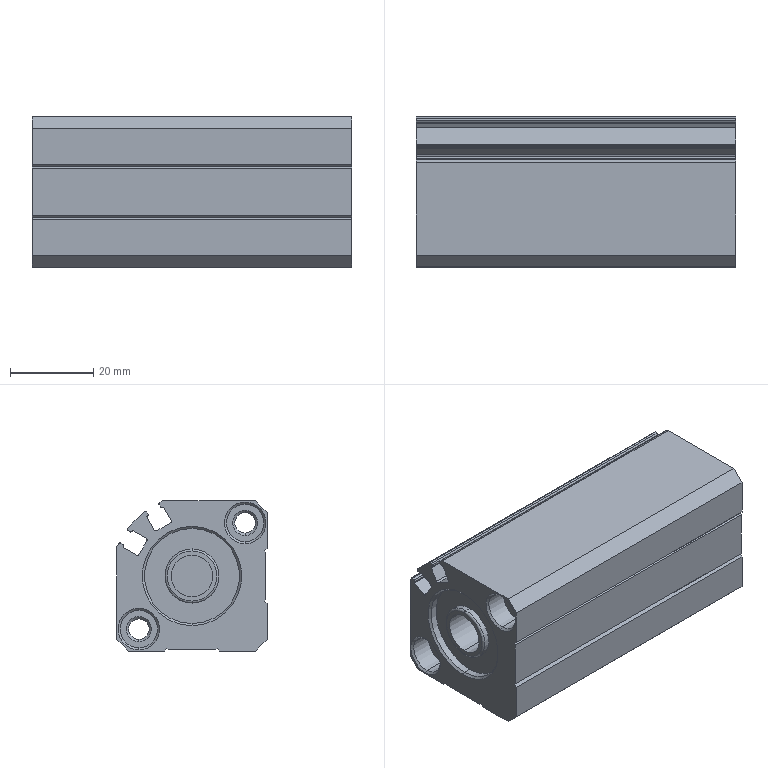Part | SolidWorks | features BaseBody 1 | 1 solid | 127 faces | box 76.5 x 36 x 36 mm | volume 64626 mm3 | cylinder 50 | plane 47 | cone 28 | torus 2 | commonest cylinder face diameters 0.8 x14 9 x8 0.4 x6 4.134 x4 4.917 x4 13 x4